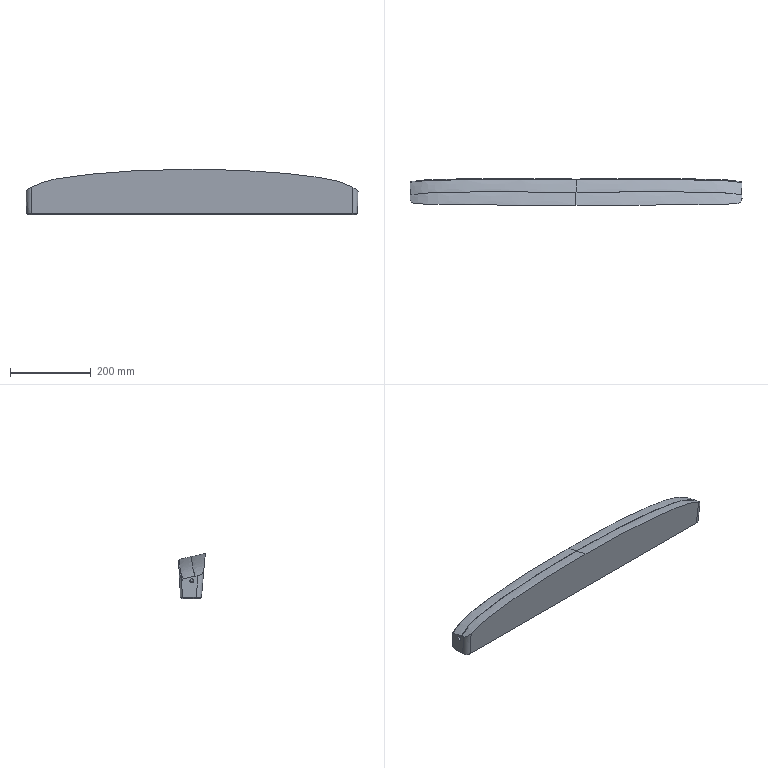Part | STEP file | solid 248 | 1 solid | 138 faces | box 819.765 x 65.53 x 111.578 mm | volume 4185351 mm3 | spline 60 | cylinder 40 | plane 32 | cone 6 | commonest cylinder face diameters 10 x10 6.078 x8 10.13 x8 30 x5 12.156 x4 14 x3